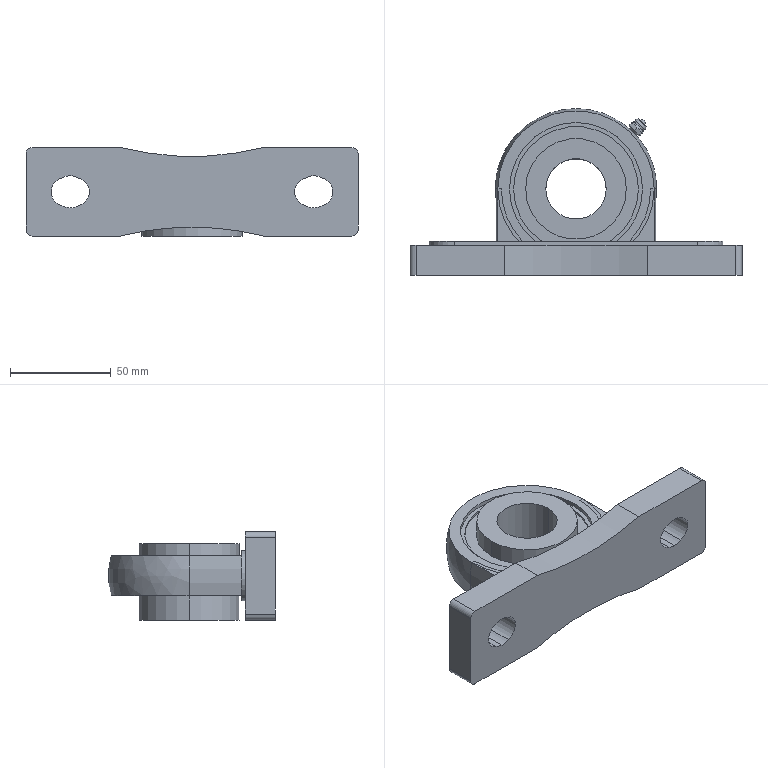Part | SolidWorks | features BaseBody 4, ICE 1 | 4 solids | 82 faces | box 165 x 83 x 44.2 mm | volume 207279 mm3 | cylinder 41 | plane 34 | spline 5 | cone 2 | commonest cylinder face diameters 16 x6 6 x4 14 x4 50.05 x4 62.08 x4 66.08 x4